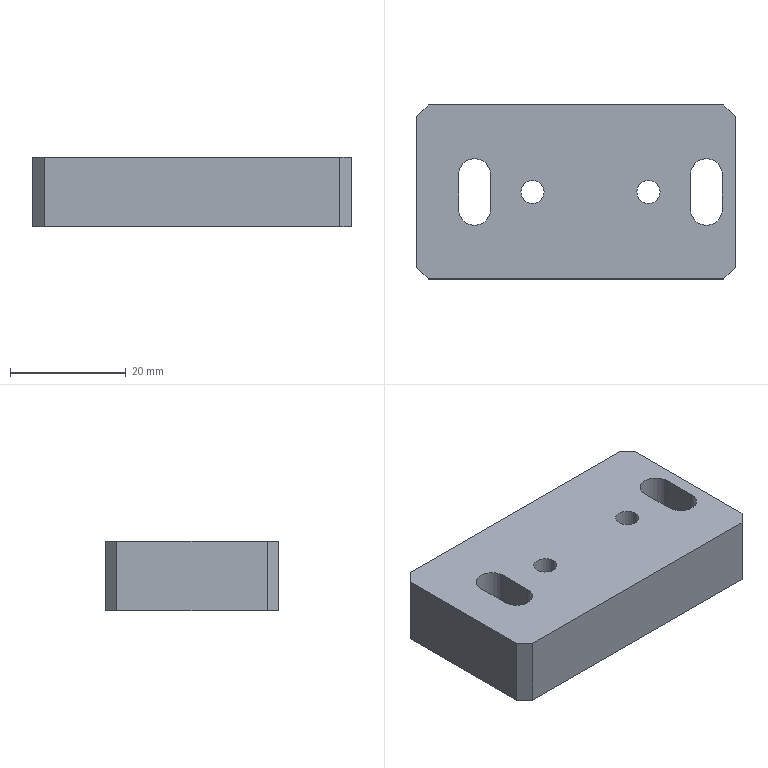Part | STEP file | 2023 Pad plate | 1 solid | 22 faces | box 55 x 30 x 12 mm | volume 18040 mm3 | plane 14 | cylinder 8 | commonest cylinder face diameters 4 x4 5.5 x4